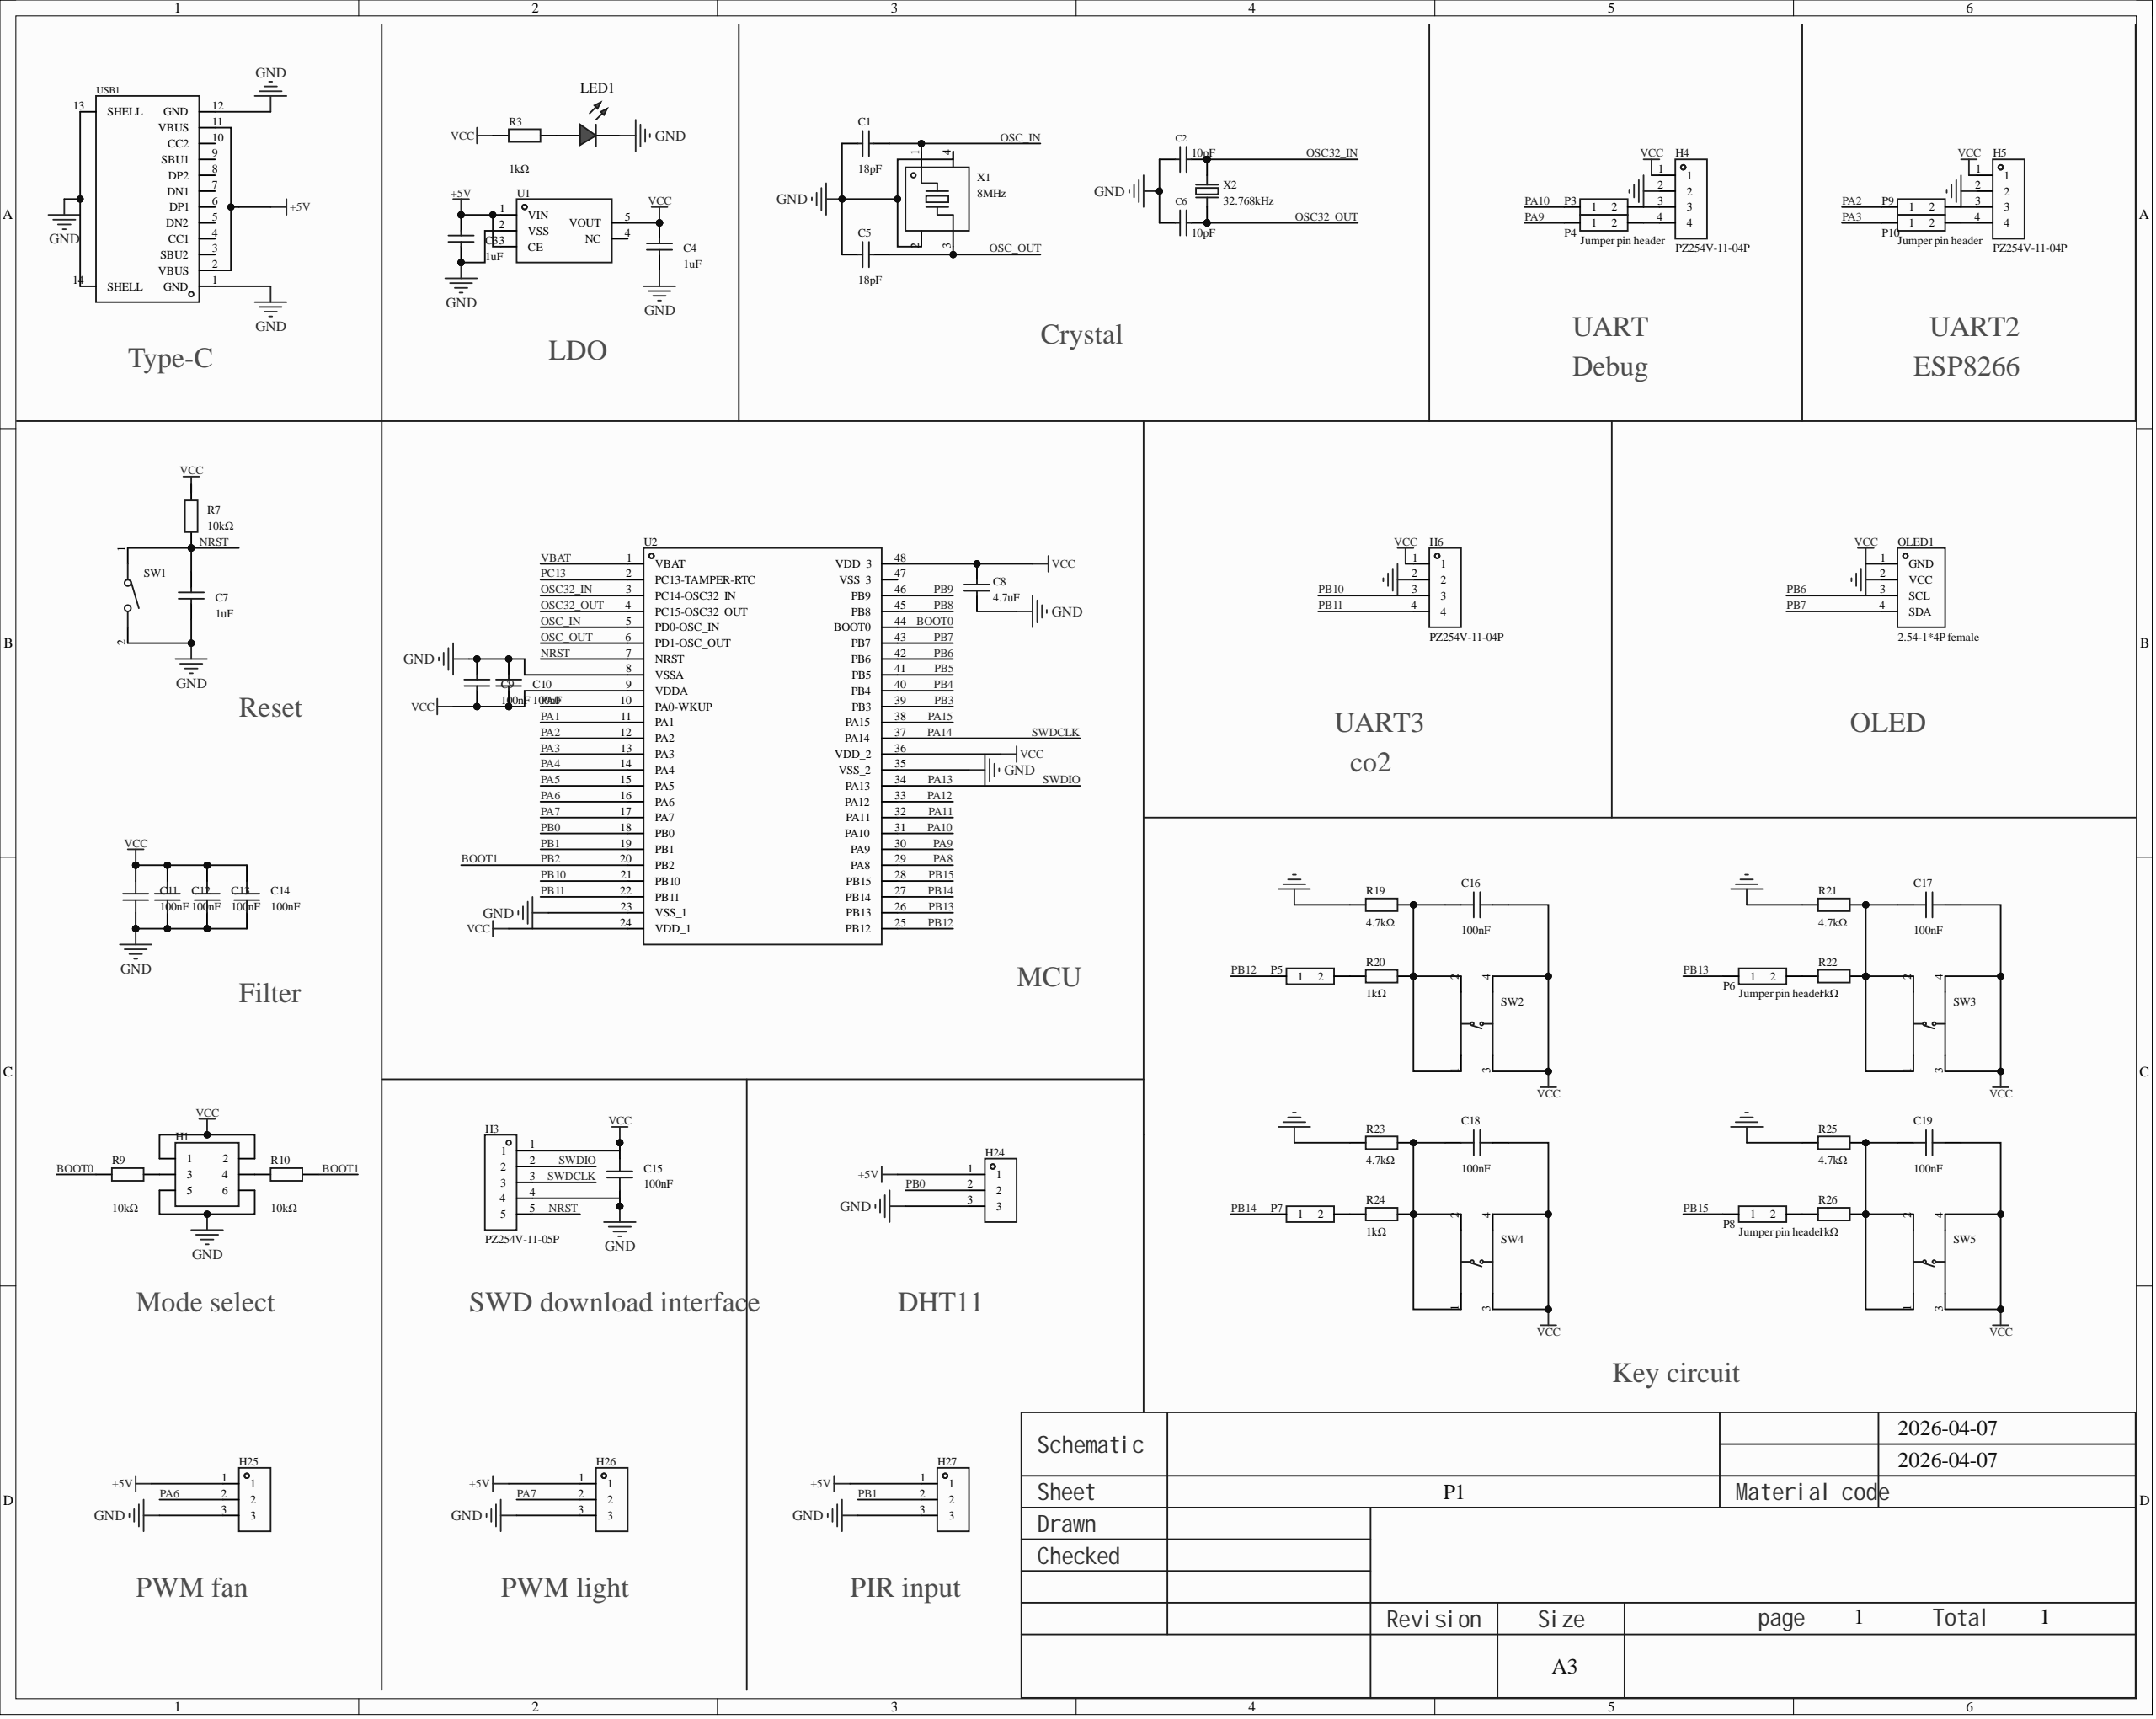Circuit board | Altium Designer | 60 parts | 43 nets
Bill of materials:
Comment,Description,Designator,Footprint,LibRef,Quantity
"FCC0603N180J500CT","Capacitance:18pF; tolerance:±5%; rated voltage:50V; temperature coefficient:C0G;","C1, C5","C0603","FCC0603N180J500CT","2"
"CL10C100JB8NNNC","Capacitance:10pF; tolerance:±5%; rated voltage:50V; temperature coefficient:C0G;","C2, C6","C0603","CL10C100JB8NNNC","2"
"CL05A105KP5NNNC","Capacitance:1uF; tolerance:±10%; rated voltage:10V; dielectric (temperature coefficient):X5R;","C3","C0603","CL05A105KP5NNNC","1"
"CL05A105KQ5NNNC","Capacitance:1uF; tolerance:±10%; rated voltage:6.3V; dielectric (temperature coefficient):X5R;","C4","C0603","CL05A105KQ5NNNC","1"
"CGA0603X5R105K500JT","Capacitance:1uF; tolerance:±10%; rated voltage:50V; temperature coefficient:X5R;","C7","C0603","CGA0603X5R105K500JT","1"
"CL10A475KO8NNNC","Capacitance:4.7uF; tolerance:±10%; rated voltage:16V; temperature coefficient:X5R;","C8","C0603","CL10A475KO8NNNC","1"
"CC0603KRX7R9BB104","Capacitance:100nF; tolerance:±10%; rated voltage:50V; temperature coefficient:X7R;","C9, C10, C11, C12, C13, C14, C15","C0603","CC0603KRX7R9BB104","7"
"100nF","Capacitance:100nF; tolerance:±10%; rated voltage:50V; temperature coefficient:X7R;","C16, C17, C18, C19","C0603","CGA0603X7R104K500JT","4"
"","","H1","HDR-TH_6P-P2.54-V-R2-C3-S2.54_A2541WV-2X3P","HDR-M_2.54_2x3","1"
"PZ254V-11-05P","","H3","HDR-TH_5P-P2.54-V-M","PZ254V-11-05P","1"
"PZ254V-11-04P","","H4, H5, H6","HDR-TH_4P-P2.54-V-M","PZ254V-11-04P","3"
"HC-PM254-8.5H-1x3PW-02A","","H24, H25, H26, H27","HDR-TH_3P-P2.54_HC-PM254-8.5H-1X3PW","HC-PM254-8.5H-1x3PW-02A","4"
"LED_0402-R","","LED1","LED_0402","LED_0402-R","1"
"2.54-1*4P female","","OLED1","HDR-TH_4P-P2.54-V-F","2.54-1*4P母","1"
"Jumper pin header","","P3, P4, P5, P6, P7, P8, P9, P10","2P排针","跳线排针-1.27mm-1×2P","8"
"0603WAF1001T5E","Resistor type:thick film resistor; resistance:1kΩ; tolerance:±1%; power:100mW; max working voltage:75V; temperature coefficient:±100ppm/?;","R3","R0603","0603WAF1001T5E","1"
"0603WAF1002T5E","Resistor type:thick film resistor; resistance:10kΩ; tolerance:±1%; power:100mW; working voltage:75V; temperature coefficient:±100ppm/?;","R7, R9, R10","R0603","0603WAF1002T5E","3"
"4.7kΩ","Resistor type:thick film resistor; resistance:4.7kΩ; tolerance:±1%; power:100mW; working voltage:75V; temperature coefficient:±100ppm/?;","R19, R21, R23, R25","R0603","0603WAF4701T5E","4"
"1kΩ","Resistor type:thick film resistor; resistance:1kΩ; tolerance:±1%; power:100mW; max working voltage:75V; temperature coefficient:±100ppm/?;","R20, R22, R24, R26","R0603","0603WAF1001T5E","4"
"TS-1088-AR02016","","SW1","SW-SMD_L3.9-W3.0-P4.45","TS-1088-AR02016","1"
"TS665CJ","Circuit:SPST; button shape:round button; mounting:through-hole; switch length:6mm; switch width:6mm; switch height:5mm; contact current:50mA; rated voltage (DC):12V; with light:-; mechanical life:-;","SW2, SW3, SW4, SW5","SW-TH_4P-L6.0-W6.0-P4.50-LS6.5","TS665CJ","4"
"ME6211C33M5G-N","Output type:fixed; output polarity:positive; max input voltage:6V; output voltage:3.3V; output current:500mA; PSRR:70dB;","U1","SOT-23-5_L3.0-W1.7-P0.95-LS2.8-BL","ME6211C33M5G-N","1"
"STM32F103C8T6","CPU core:CM3; program memory:64KB; total RAM:20KB; GPIO count:37; operating voltage range:2V~3.6V; max CPU frequency:72MHz; program memory type:FLASH;","U2","LQFP-48_L7.0-W7.0-P0.50-LS9.0-BL","STM32F103C8T6","1"
"TYPE-C 16PIN 2MD(073)","","USB1","USB-C-SMD_TYPE-C-6PIN-2MD-073","TYPE-C 16PIN 2MD(073)","1"
"8MHz","Crystal type:SMD crystal; frequency:8MHz; room-temperature frequency tolerance:±10ppm; load capacitance:12pF; frequency stability (full temperature):±20ppm;","X1","OSC-SMD_4P-L3.2-W2.5-BL","X32258MOB4SI","1"
"Q13FC13500049","Crystal type:SMD crystal; frequency:32.768kHz; room-temperature frequency tolerance:±20ppm; load capacitance:6pF;","X2","CRYSTAL-SMD_L3.2-W1.5-1","Q13FC13500049","1"
Netlist (Protel format):
[
C1
C0603
FCC0603N180J500CT



]
[
C2
C0603
CL10C100JB8NNNC



]
[
C3
C0603
CL05A105KP5NNNC



]
[
C4
C0603
CL05A105KQ5NNNC



]
[
C5
C0603
FCC0603N180J500CT



]
[
C6
C0603
CL10C100JB8NNNC



]
[
C7
C0603
CGA0603X5R105K500JT



]
[
C8
C0603
CL10A475KO8NNNC



]
[
C9
C0603
CC0603KRX7R9BB104



]
[
C10
C0603
CC0603KRX7R9BB104



]
[
C11
C0603
CC0603KRX7R9BB104



]
[
C12
C0603
CC0603KRX7R9BB104



]
[
C13
C0603
CC0603KRX7R9BB104



]
[
C14
C0603
CC0603KRX7R9BB104



]
[
C15
C0603
CC0603KRX7R9BB104



]
[
C16
C0603
100nF



]
[
C17
C0603
100nF



]
[
C18
C0603
100nF



]
[
C19
C0603
100nF



]
[
H1
HDR-TH_6P-P2.54-V-R2-C3-S2.54_A2541WV-2X3P




]
[
H3
HDR-TH_5P-P2.54-V-M
PZ254V-11-05P



]
[
H4
HDR-TH_4P-P2.54-V-M
PZ254V-11-04P



]
[
H5
HDR-TH_4P-P2.54-V-M
PZ254V-11-04P



]
[
H6
HDR-TH_4P-P2.54-V-M
PZ254V-11-04P



]
[
H24
HDR-TH_3P-P2.54_HC-PM254-8.5H-1X3PW
HC-PM254-8.5H-1x3PW-02A



]
[
H25
HDR-TH_3P-P2.54_HC-PM254-8.5H-1X3PW
HC-PM254-8.5H-1x3PW-02A



]
[
H26
HDR-TH_3P-P2.54_HC-PM254-8.5H-1X3PW
HC-PM254-8.5H-1x3PW-02A



]
[
H27
HDR-TH_3P-P2.54_HC-PM254-8.5H-1X3PW
HC-PM254-8.5H-1x3PW-02A



]
[
LED1
LED_0402
LED_0402-R



]
[
OLED1
HDR-TH_4P-P2.54-V-F
2.54-1*4P female



]
[
P3
2P排针
Jumper pin header



]
[
P4
2P排针
Jumper pin header



]
[
P5
2P排针
Jumper pin header



]
[
P6
2P排针
Jumper pin header



]
[
P7
2P排针
Jumper pin header



]
[
P8
2P排针
Jumper pin header



]
[
P9
2P排针
Jumper pin header



]
[
P10
2P排针
Jumper pin header



]
[
R3
R0603
0603WAF1001T5E



]
[
R7
R0603
0603WAF1002T5E



]
[
R9
R0603
0603WAF1002T5E



]
[
R10
R0603
0603WAF1002T5E



]
[
R19
R0603
4.7kΩ



]
[
R20
R0603
1kΩ



]
[
R21
R0603
4.7kΩ



]
[
R22
R0603
1kΩ



]
[
R23
R0603
4.7kΩ



]
[
R24
R0603
1kΩ



]
[
R25
R0603
4.7kΩ



]
[
R26
R0603
1kΩ



]
[
SW1
SW-SMD_L3.9-W3.0-P4.45
TS-1088-AR02016



]
[
SW2
SW-TH_4P-L6.0-W6.0-P4.50-LS6.5
TS665CJ



]
[
SW3
SW-TH_4P-L6.0-W6.0-P4.50-LS6.5
TS665CJ



]
[
SW4
SW-TH_4P-L6.0-W6.0-P4.50-LS6.5
TS665CJ



]
[
SW5
SW-TH_4P-L6.0-W6.0-P4.50-LS6.5
TS665CJ



]
[
U1
SOT-23-5_L3.0-W1.7-P0.95-LS2.8-BL
ME6211C33M5G-N



]
[
U2
LQFP-48_L7.0-W7.0-P0.50-LS9.0-BL
STM32F103C8T6



]
[
USB1
USB-C-SMD_TYPE-C-6PIN-2MD-073
TYPE-C 16PIN 2MD(073)



]
[
X1
OSC-SMD_4P-L3.2-W2.5-BL
8MHz



]
[
X2
CRYSTAL-SMD_L3.2-W1.5-1
Q13FC13500049



]
(
VCC
C4-2
C8-2
C9-1
C10-1
C11-2
C12-2
C13-2
C14-2
C15-2
C16-2
C17-2
C18-2
C19-2
H1-1
H1-2
H3-1
H4-1
H5-1
H6-1
OLED1-1
R3-1
R7-2
SW2-3
SW2-4
SW3-3
SW3-4
SW4-3
SW4-4
SW5-3
SW5-4
U1-5
U2-9
U2-24
U2-36
U2-48
)
(
PB15
P8-1
U2-28
)
(
PB14
P7-1
U2-27
)
(
PB13
P6-1
U2-26
)
(
PB12
P5-1
U2-25
)
(
PB11
H6-4
U2-22
)
(
PB10
H6-3
U2-21
)
(
PB7
OLED1-4
U2-43
)
(
PB6
OLED1-3
U2-42
)
(
PB1
H27-2
U2-19
)
(
PB0
H24-2
U2-18
)
(
PA14
H3-3
U2-37
)
(
PA13
H3-2
U2-34
)
(
PA10
P3-1
U2-31
)
(
PA9
P4-1
U2-30
)
(
PA7
H26-2
U2-17
)
(
PA6
H25-2
U2-16
)
(
PA3
P10-1
U2-13
)
(
PA2
P9-1
U2-12
)
(
OSC_OUT
C5-1
U2-6
X1-3
)
(
OSC_IN
C1-1
U2-5
X1-1
)
(
OSC32_OUT
C6-2
U2-4
X2-1
)
(
OSC32_IN
C2-2
U2-3
X2-2
)
(
NRST
C7-1
H3-5
R7-1
SW1-1
U2-7
)
(
NetP8_2
P8-2
R26-1
)
(
NetP7_2
P7-2
R24-1
)
(
NetP6_2
P6-2
R22-1
)
(
NetP5_2
P5-2
R20-1
)
(
NetLED1_2
LED1-2
R3-2
)
(
NetH5_4
H5-4
P10-2
)
(
NetH5_3
H5-3
P9-2
)
(
NetH4_4
H4-4
P4-2
)
(
NetH4_3
H4-3
P3-2
)
(
NetH1_4
H1-4
R10-1
)
(
NetH1_3
H1-3
R9-2
)
(
NetC19_1
C19-1
R25-2
R26-2
SW5-1
SW5-2
)
(
NetC18_1
C18-1
R23-2
R24-2
SW4-1
SW4-2
)
(
NetC17_1
C17-1
R21-2
R22-2
SW3-1
SW3-2
)
(
NetC16_1
C16-1
R19-2
R20-2
SW2-1
SW2-2
)
(
GND
C1-2
C2-1
C3-1
C4-1
C5-2
C6-1
C7-2
C8-1
C9-2
C10-2
C11-1
C12-1
C13-1
C14-1
C15-1
H1-5
H1-6
H3-4
H4-2
H5-2
H6-2
H24-3
H25-3
H26-3
H27-3
LED1-1
OLED1-2
R19-1
R21-1
R23-1
R25-1
SW1-2
U1-2
U2-8
U2-23
U2-35
USB1-1
USB1-12
USB1-13
USB1-14
X1-2
X1-4
)
(
BOOT1
R10-2
U2-20
)
(
BOOT0
R9-1
U2-44
)
(
+5V
C3-2
H24-1
H25-1
H26-1
H27-1
U1-1
U1-3
USB1-2
USB1-11
)